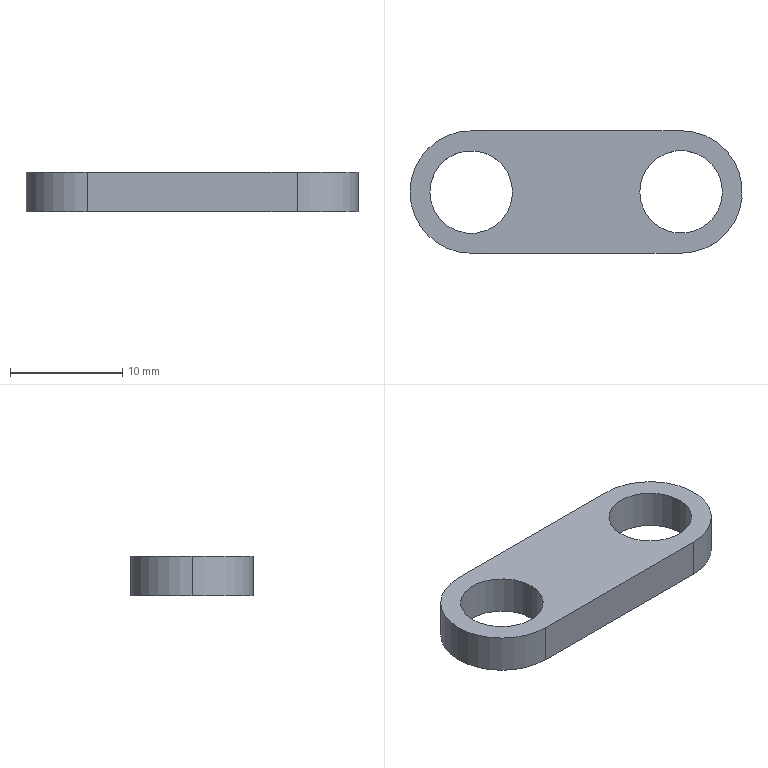Part | SolidWorks | features Extrusion 1 | 1 solid | 11 faces | box 29.554 x 10.9 x 3.5 mm | volume 740.438 mm3 | cylinder 7 | plane 4 | commonest cylinder face diameters 7.349 x4 10.89 x3
STEP:
#1=CARTESIAN_POINT('',(2.019,0.007713,3.5));
#2=VERTEX_POINT('',#1);
#3=CARTESIAN_POINT('',(7.464,-5.437,3.5));
#4=VERTEX_POINT('',#3);
#5=CARTESIAN_POINT('',(7.464,0.007713,3.5));
#6=DIRECTION('',(0.,0.,1.));
#7=DIRECTION('',(1.,0.,0.));
#8=AXIS2_PLACEMENT_3D('',#5,#6,#7);
#9=CIRCLE('',#8,5.445);
#10=EDGE_CURVE('',#2,#4,#9,.T.);
#11=ORIENTED_EDGE('',*,*,#10,.F.);
#12=CARTESIAN_POINT('',(2.019,0.007713,0.));
#13=VERTEX_POINT('',#12);
#14=CARTESIAN_POINT('',(2.019,0.007713,35.));
#15=DIRECTION('',(0.,0.,-1.));
#16=VECTOR('',#15,1000.);
#17=LINE('',#14,#16);
#18=EDGE_CURVE('',#2,#13,#17,.T.);
#19=ORIENTED_EDGE('',*,*,#18,.T.);
#20=CARTESIAN_POINT('',(7.464,-5.437,0.));
#21=VERTEX_POINT('',#20);
#22=CARTESIAN_POINT('',(7.464,0.007713,0.));
#23=DIRECTION('',(0.,0.,1.));
#24=DIRECTION('',(1.,0.,0.));
#25=AXIS2_PLACEMENT_3D('',#22,#23,#24);
#26=CIRCLE('',#25,5.445);
#27=EDGE_CURVE('',#13,#21,#26,.T.);
#28=ORIENTED_EDGE('',*,*,#27,.T.);
#29=CARTESIAN_POINT('',(7.464,-5.437,35.));
#30=DIRECTION('',(0.,0.,-1.));
#31=VECTOR('',#30,1000.);
#32=LINE('',#29,#31);
#33=EDGE_CURVE('',#4,#21,#32,.T.);
#34=ORIENTED_EDGE('',*,*,#33,.F.);
#35=EDGE_LOOP('',(#11,#19,#28,#34));
#36=FACE_OUTER_BOUND('',#35,.T.);
#37=CARTESIAN_POINT('',(7.464,0.007713,35.));
#38=DIRECTION('',(0.,0.,-1.));
#39=DIRECTION('',(-1.,0.,0.));
#40=AXIS2_PLACEMENT_3D('',#37,#38,#39);
#41=CYLINDRICAL_SURFACE('',#40,5.445);
#42=ADVANCED_FACE('',(#36),#41,.T.);
#43=CARTESIAN_POINT('',(3.789,0.007713,3.5));
#44=VERTEX_POINT('',#43);
#45=CARTESIAN_POINT('',(11.139,0.007713,3.5));
#46=VERTEX_POINT('',#45);
#47=CARTESIAN_POINT('',(7.464,0.007713,3.5));
#48=DIRECTION('',(0.,0.,1.));
#49=DIRECTION('',(1.,0.,0.));
#50=AXIS2_PLACEMENT_3D('',#47,#48,#49);
#51=CIRCLE('',#50,3.675);
#52=EDGE_CURVE('',#44,#46,#51,.T.);
#53=ORIENTED_EDGE('',*,*,#52,.T.);
#54=CARTESIAN_POINT('',(11.139,0.007713,0.));
#55=VERTEX_POINT('',#54);
#56=CARTESIAN_POINT('',(11.139,0.007713,35.));
#57=DIRECTION('',(0.,0.,-1.));
#58=VECTOR('',#57,1000.);
#59=LINE('',#56,#58);
#60=EDGE_CURVE('',#46,#55,#59,.T.);
#61=ORIENTED_EDGE('',*,*,#60,.T.);
#62=CARTESIAN_POINT('',(3.789,0.007713,0.));
#63=VERTEX_POINT('',#62);
#64=CARTESIAN_POINT('',(7.464,0.007713,0.));
#65=DIRECTION('',(0.,0.,1.));
#66=DIRECTION('',(1.,0.,0.));
#67=AXIS2_PLACEMENT_3D('',#64,#65,#66);
#68=CIRCLE('',#67,3.675);
#69=EDGE_CURVE('',#63,#55,#68,.T.);
#70=ORIENTED_EDGE('',*,*,#69,.F.);
#71=CARTESIAN_POINT('',(3.789,0.007713,35.));
#72=DIRECTION('',(0.,0.,-1.));
#73=VECTOR('',#72,1000.);
#74=LINE('',#71,#73);
#75=EDGE_CURVE('',#44,#63,#74,.T.);
#76=ORIENTED_EDGE('',*,*,#75,.F.);
#77=EDGE_LOOP('',(#53,#61,#70,#76));
#78=FACE_OUTER_BOUND('',#77,.T.);
#79=CARTESIAN_POINT('',(7.464,0.007713,35.));
#80=DIRECTION('',(0.,0.,-1.));
#81=DIRECTION('',(-1.,0.,0.));
#82=AXIS2_PLACEMENT_3D('',#79,#80,#81);
#83=CYLINDRICAL_SURFACE('',#82,3.675);
#84=ADVANCED_FACE('',(#78),#83,.F.);
#85=CARTESIAN_POINT('',(22.454,0.01736,3.5));
#86=VERTEX_POINT('',#85);
#87=CARTESIAN_POINT('',(29.803,0.01736,3.5));
#88=VERTEX_POINT('',#87);
#89=CARTESIAN_POINT('',(26.128,0.01736,3.5));
#90=DIRECTION('',(0.,0.,1.));
#91=DIRECTION('',(1.,0.,0.));
#92=AXIS2_PLACEMENT_3D('',#89,#90,#91);
#93=CIRCLE('',#92,3.675);
#94=EDGE_CURVE('',#86,#88,#93,.T.);
#95=ORIENTED_EDGE('',*,*,#94,.T.);
#96=CARTESIAN_POINT('',(29.803,0.01736,0.));
#97=VERTEX_POINT('',#96);
#98=CARTESIAN_POINT('',(29.803,0.01736,35.));
#99=DIRECTION('',(0.,0.,-1.));
#100=VECTOR('',#99,1000.);
#101=LINE('',#98,#100);
#102=EDGE_CURVE('',#88,#97,#101,.T.);
#103=ORIENTED_EDGE('',*,*,#102,.T.);
#104=CARTESIAN_POINT('',(22.454,0.01736,0.));
#105=VERTEX_POINT('',#104);
#106=CARTESIAN_POINT('',(26.128,0.01736,0.));
#107=DIRECTION('',(0.,0.,1.));
#108=DIRECTION('',(1.,0.,0.));
#109=AXIS2_PLACEMENT_3D('',#106,#107,#108);
#110=CIRCLE('',#109,3.675);
#111=EDGE_CURVE('',#105,#97,#110,.T.);
#112=ORIENTED_EDGE('',*,*,#111,.F.);
#113=CARTESIAN_POINT('',(22.454,0.01736,35.));
#114=DIRECTION('',(0.,0.,-1.));
#115=VECTOR('',#114,1000.);
#116=LINE('',#113,#115);
#117=EDGE_CURVE('',#86,#105,#116,.T.);
#118=ORIENTED_EDGE('',*,*,#117,.F.);
#119=EDGE_LOOP('',(#95,#103,#112,#118));
#120=FACE_OUTER_BOUND('',#119,.T.);
#121=CARTESIAN_POINT('',(26.128,0.01736,35.));
#122=DIRECTION('',(0.,0.,-1.));
#123=DIRECTION('',(-1.,0.,0.));
#124=AXIS2_PLACEMENT_3D('',#121,#122,#123);
#125=CYLINDRICAL_SURFACE('',#124,3.675);
#126=ADVANCED_FACE('',(#120),#125,.F.);
#127=CARTESIAN_POINT('',(26.128,-5.428,3.5));
#128=VERTEX_POINT('',#127);
#129=CARTESIAN_POINT('',(0.002811,-5.441,3.5));
#130=DIRECTION('',(1.,0.0005166,0.));
#131=VECTOR('',#130,1000.);
#132=LINE('',#129,#131);
#133=EDGE_CURVE('',#4,#128,#132,.T.);
#134=ORIENTED_EDGE('',*,*,#133,.F.);
#135=ORIENTED_EDGE('',*,*,#33,.T.);
#136=CARTESIAN_POINT('',(26.128,-5.428,0.));
#137=VERTEX_POINT('',#136);
#138=CARTESIAN_POINT('',(0.002811,-5.441,0.));
#139=DIRECTION('',(1.,0.0005166,0.));
#140=VECTOR('',#139,1000.);
#141=LINE('',#138,#140);
#142=EDGE_CURVE('',#21,#137,#141,.T.);
#143=ORIENTED_EDGE('',*,*,#142,.T.);
#144=CARTESIAN_POINT('',(26.128,-5.428,35.));
#145=DIRECTION('',(0.,0.,-1.));
#146=VECTOR('',#145,1000.);
#147=LINE('',#144,#146);
#148=EDGE_CURVE('',#128,#137,#147,.T.);
#149=ORIENTED_EDGE('',*,*,#148,.F.);
#150=EDGE_LOOP('',(#134,#135,#143,#149));
#151=FACE_OUTER_BOUND('',#150,.T.);
#152=CARTESIAN_POINT('',(0.002811,-5.441,35.));
#153=DIRECTION('',(-0.0005166,1.,0.));
#154=DIRECTION('',(-1.,-0.0005166,0.));
#155=AXIS2_PLACEMENT_3D('',#152,#153,#154);
#156=PLANE('',#155);
#157=ADVANCED_FACE('',(#151),#156,.F.);
#158=CARTESIAN_POINT('',(26.125,5.462,3.5));
#159=VERTEX_POINT('',#158);
#160=CARTESIAN_POINT('',(26.128,0.01736,3.5));
#161=DIRECTION('',(0.,0.,1.));
#162=DIRECTION('',(1.,0.,0.));
#163=AXIS2_PLACEMENT_3D('',#160,#161,#162);
#164=CIRCLE('',#163,5.445);
#165=EDGE_CURVE('',#128,#159,#164,.T.);
#166=ORIENTED_EDGE('',*,*,#165,.F.);
#167=ORIENTED_EDGE('',*,*,#148,.T.);
#168=CARTESIAN_POINT('',(26.125,5.462,0.));
#169=VERTEX_POINT('',#168);
#170=CARTESIAN_POINT('',(26.128,0.01736,0.));
#171=DIRECTION('',(0.,0.,1.));
#172=DIRECTION('',(1.,0.,0.));
#173=AXIS2_PLACEMENT_3D('',#170,#171,#172);
#174=CIRCLE('',#173,5.445);
#175=EDGE_CURVE('',#137,#169,#174,.T.);
#176=ORIENTED_EDGE('',*,*,#175,.T.);
#177=CARTESIAN_POINT('',(26.125,5.462,35.));
#178=DIRECTION('',(0.,0.,-1.));
#179=VECTOR('',#178,1000.);
#180=LINE('',#177,#179);
#181=EDGE_CURVE('',#159,#169,#180,.T.);
#182=ORIENTED_EDGE('',*,*,#181,.F.);
#183=EDGE_LOOP('',(#166,#167,#176,#182));
#184=FACE_OUTER_BOUND('',#183,.T.);
#185=CARTESIAN_POINT('',(26.128,0.01736,35.));
#186=DIRECTION('',(0.,0.,-1.));
#187=DIRECTION('',(-1.,0.,0.));
#188=AXIS2_PLACEMENT_3D('',#185,#186,#187);
#189=CYLINDRICAL_SURFACE('',#188,5.445);
#190=ADVANCED_FACE('',(#184),#189,.T.);
#191=CARTESIAN_POINT('',(7.464,5.453,3.5));
#192=VERTEX_POINT('',#191);
#193=CARTESIAN_POINT('',(7.464,5.453,0.));
#194=VERTEX_POINT('',#193);
#195=CARTESIAN_POINT('',(7.464,5.453,35.));
#196=DIRECTION('',(0.,0.,-1.));
#197=VECTOR('',#196,1000.);
#198=LINE('',#195,#197);
#199=EDGE_CURVE('',#192,#194,#198,.T.);
#200=ORIENTED_EDGE('',*,*,#199,.F.);
#201=CARTESIAN_POINT('',(-0.002815,5.449,3.5));
#202=DIRECTION('',(1.,0.0005167,0.));
#203=VECTOR('',#202,1000.);
#204=LINE('',#201,#203);
#205=EDGE_CURVE('',#192,#159,#204,.T.);
#206=ORIENTED_EDGE('',*,*,#205,.T.);
#207=ORIENTED_EDGE('',*,*,#181,.T.);
#208=CARTESIAN_POINT('',(-0.002815,5.449,0.));
#209=DIRECTION('',(1.,0.0005167,0.));
#210=VECTOR('',#209,1000.);
#211=LINE('',#208,#210);
#212=EDGE_CURVE('',#194,#169,#211,.T.);
#213=ORIENTED_EDGE('',*,*,#212,.F.);
#214=EDGE_LOOP('',(#200,#206,#207,#213));
#215=FACE_OUTER_BOUND('',#214,.T.);
#216=CARTESIAN_POINT('',(-0.002815,5.449,35.));
#217=DIRECTION('',(-0.0005167,1.,0.));
#218=DIRECTION('',(-1.,-0.0005167,0.));
#219=AXIS2_PLACEMENT_3D('',#216,#217,#218);
#220=PLANE('',#219);
#221=ADVANCED_FACE('',(#215),#220,.T.);
#222=ORIENTED_EDGE('',*,*,#102,.F.);
#223=CARTESIAN_POINT('',(26.128,0.01736,3.5));
#224=DIRECTION('',(0.,0.,1.));
#225=DIRECTION('',(1.,0.,0.));
#226=AXIS2_PLACEMENT_3D('',#223,#224,#225);
#227=CIRCLE('',#226,3.675);
#228=EDGE_CURVE('',#88,#86,#227,.T.);
#229=ORIENTED_EDGE('',*,*,#228,.T.);
#230=ORIENTED_EDGE('',*,*,#117,.T.);
#231=CARTESIAN_POINT('',(26.128,0.01736,0.));
#232=DIRECTION('',(0.,0.,1.));
#233=DIRECTION('',(1.,0.,0.));
#234=AXIS2_PLACEMENT_3D('',#231,#232,#233);
#235=CIRCLE('',#234,3.675);
#236=EDGE_CURVE('',#97,#105,#235,.T.);
#237=ORIENTED_EDGE('',*,*,#236,.F.);
#238=EDGE_LOOP('',(#222,#229,#230,#237));
#239=FACE_OUTER_BOUND('',#238,.T.);
#240=CARTESIAN_POINT('',(26.128,0.01736,35.));
#241=DIRECTION('',(0.,0.,-1.));
#242=DIRECTION('',(-1.,0.,0.));
#243=AXIS2_PLACEMENT_3D('',#240,#241,#242);
#244=CYLINDRICAL_SURFACE('',#243,3.675);
#245=ADVANCED_FACE('',(#239),#244,.F.);
#246=ORIENTED_EDGE('',*,*,#60,.F.);
#247=CARTESIAN_POINT('',(7.464,0.007713,3.5));
#248=DIRECTION('',(0.,0.,1.));
#249=DIRECTION('',(1.,0.,0.));
#250=AXIS2_PLACEMENT_3D('',#247,#248,#249);
#251=CIRCLE('',#250,3.675);
#252=EDGE_CURVE('',#46,#44,#251,.T.);
#253=ORIENTED_EDGE('',*,*,#252,.T.);
#254=ORIENTED_EDGE('',*,*,#75,.T.);
#255=CARTESIAN_POINT('',(7.464,0.007713,0.));
#256=DIRECTION('',(0.,0.,1.));
#257=DIRECTION('',(1.,0.,0.));
#258=AXIS2_PLACEMENT_3D('',#255,#256,#257);
#259=CIRCLE('',#258,3.675);
#260=EDGE_CURVE('',#55,#63,#259,.T.);
#261=ORIENTED_EDGE('',*,*,#260,.F.);
#262=EDGE_LOOP('',(#246,#253,#254,#261));
#263=FACE_OUTER_BOUND('',#262,.T.);
#264=CARTESIAN_POINT('',(7.464,0.007713,35.));
#265=DIRECTION('',(0.,0.,-1.));
#266=DIRECTION('',(-1.,0.,0.));
#267=AXIS2_PLACEMENT_3D('',#264,#265,#266);
#268=CYLINDRICAL_SURFACE('',#267,3.675);
#269=ADVANCED_FACE('',(#263),#268,.F.);
#270=ORIENTED_EDGE('',*,*,#18,.F.);
#271=CARTESIAN_POINT('',(7.464,0.007713,3.5));
#272=DIRECTION('',(0.,0.,1.));
#273=DIRECTION('',(1.,0.,0.));
#274=AXIS2_PLACEMENT_3D('',#271,#272,#273);
#275=CIRCLE('',#274,5.445);
#276=EDGE_CURVE('',#192,#2,#275,.T.);
#277=ORIENTED_EDGE('',*,*,#276,.F.);
#278=ORIENTED_EDGE('',*,*,#199,.T.);
#279=CARTESIAN_POINT('',(7.464,0.007713,0.));
#280=DIRECTION('',(0.,0.,1.));
#281=DIRECTION('',(1.,0.,0.));
#282=AXIS2_PLACEMENT_3D('',#279,#280,#281);
#283=CIRCLE('',#282,5.445);
#284=EDGE_CURVE('',#194,#13,#283,.T.);
#285=ORIENTED_EDGE('',*,*,#284,.T.);
#286=EDGE_LOOP('',(#270,#277,#278,#285));
#287=FACE_OUTER_BOUND('',#286,.T.);
#288=CARTESIAN_POINT('',(7.464,0.007713,35.));
#289=DIRECTION('',(0.,0.,-1.));
#290=DIRECTION('',(-1.,0.,0.));
#291=AXIS2_PLACEMENT_3D('',#288,#289,#290);
#292=CYLINDRICAL_SURFACE('',#291,5.445);
#293=ADVANCED_FACE('',(#287),#292,.T.);
#294=ORIENTED_EDGE('',*,*,#69,.T.);
#295=ORIENTED_EDGE('',*,*,#260,.T.);
#296=EDGE_LOOP('',(#294,#295));
#297=FACE_BOUND('',#296,.T.);
#298=ORIENTED_EDGE('',*,*,#111,.T.);
#299=ORIENTED_EDGE('',*,*,#236,.T.);
#300=EDGE_LOOP('',(#298,#299));
#301=FACE_BOUND('',#300,.T.);
#302=ORIENTED_EDGE('',*,*,#142,.F.);
#303=ORIENTED_EDGE('',*,*,#27,.F.);
#304=ORIENTED_EDGE('',*,*,#284,.F.);
#305=ORIENTED_EDGE('',*,*,#212,.T.);
#306=ORIENTED_EDGE('',*,*,#175,.F.);
#307=EDGE_LOOP('',(#302,#303,#304,#305,#306));
#308=FACE_OUTER_BOUND('',#307,.T.);
#309=CARTESIAN_POINT('',(0.,0.,0.));
#310=DIRECTION('',(0.,0.,1.));
#311=DIRECTION('',(1.,0.,0.));
#312=AXIS2_PLACEMENT_3D('',#309,#310,#311);
#313=PLANE('',#312);
#314=ADVANCED_FACE('',(#297,#301,#308),#313,.F.);
#315=ORIENTED_EDGE('',*,*,#94,.F.);
#316=ORIENTED_EDGE('',*,*,#228,.F.);
#317=EDGE_LOOP('',(#315,#316));
#318=FACE_BOUND('',#317,.T.);
#319=ORIENTED_EDGE('',*,*,#52,.F.);
#320=ORIENTED_EDGE('',*,*,#252,.F.);
#321=EDGE_LOOP('',(#319,#320));
#322=FACE_BOUND('',#321,.T.);
#323=ORIENTED_EDGE('',*,*,#276,.T.);
#324=ORIENTED_EDGE('',*,*,#10,.T.);
#325=ORIENTED_EDGE('',*,*,#133,.T.);
#326=ORIENTED_EDGE('',*,*,#165,.T.);
#327=ORIENTED_EDGE('',*,*,#205,.F.);
#328=EDGE_LOOP('',(#323,#324,#325,#326,#327));
#329=FACE_OUTER_BOUND('',#328,.T.);
#330=CARTESIAN_POINT('',(27.066,16.289,3.5));
#331=DIRECTION('',(0.,0.,1.));
#332=DIRECTION('',(0.9983,-0.05755,0.));
#333=AXIS2_PLACEMENT_3D('',#330,#331,#332);
#334=PLANE('',#333);
#335=ADVANCED_FACE('',(#318,#322,#329),#334,.T.);
#336=CLOSED_SHELL('',(#42,#84,#126,#157,#190,#221,#245,#269,#293,#314,#335));
#337=MANIFOLD_SOLID_BREP('',#336);
#338=CARTESIAN_POINT('',(0.,0.,0.));
#339=DIRECTION('',(0.,0.,1.));
#340=DIRECTION('',(1.,0.,0.));
#341=AXIS2_PLACEMENT_3D('',#338,#339,#340);
#342=(LENGTH_UNIT()NAMED_UNIT(*)SI_UNIT(.MILLI.,.METRE.));
#343=UNCERTAINTY_MEASURE_WITH_UNIT(LENGTH_MEASURE(0.00001),#342,'','');
#344=(NAMED_UNIT(*)PLANE_ANGLE_UNIT()SI_UNIT($,.RADIAN.));
#345=(NAMED_UNIT(*)SI_UNIT($,.STERADIAN.)SOLID_ANGLE_UNIT());
#346=(GEOMETRIC_REPRESENTATION_CONTEXT(3)GLOBAL_UNCERTAINTY_ASSIGNED_CONTEXT((#343))GLOBAL_UNIT_ASSIGNED_CONTEXT((#342,#344,#345))REPRESENTATION_CONTEXT('',''));
#347=ADVANCED_BREP_SHAPE_REPRESENTATION('',(#337,#341),#346);